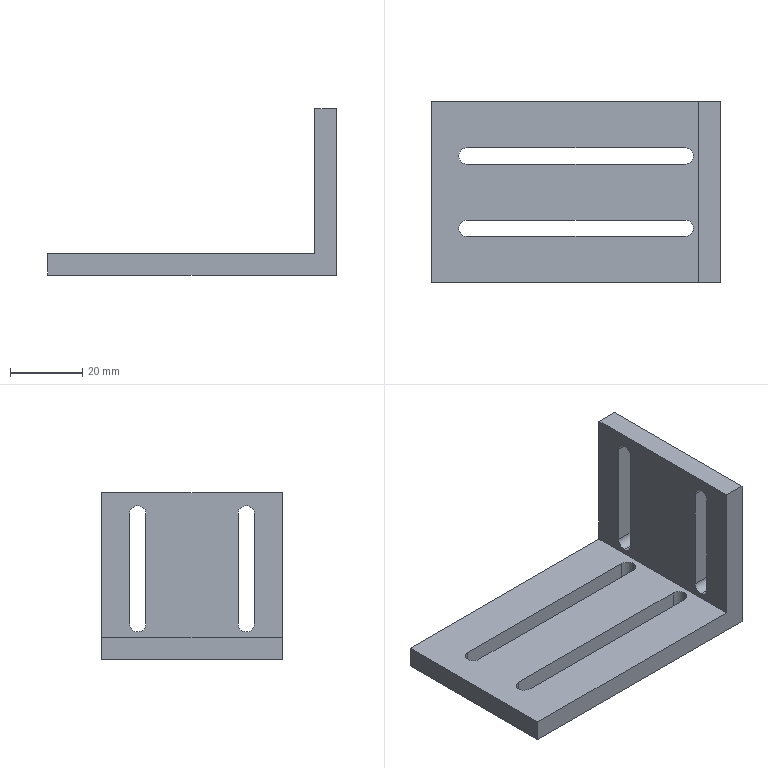Part | SolidWorks | features HoleWzd 2, Extrusion 1, ICE 1 | 1 solid | 28 faces | box 80 x 50 x 46 mm | volume 30704 mm3 | plane 16 | cylinder 12 | commonest cylinder face diameters 4.5 x12
STEP:
#1=CARTESIAN_POINT('',(34.,-15.,7.5));
#2=VERTEX_POINT('',#1);
#3=CARTESIAN_POINT('',(34.,-12.75,9.75));
#4=VERTEX_POINT('',#3);
#5=CARTESIAN_POINT('',(34.,-15.,9.75));
#6=DIRECTION('',(1.,0.,0.));
#7=DIRECTION('',(0.,0.,-1.));
#8=AXIS2_PLACEMENT_3D('',#5,#6,#7);
#9=CIRCLE('',#8,2.25);
#10=EDGE_CURVE('',#2,#4,#9,.T.);
#11=ORIENTED_EDGE('',*,*,#10,.F.);
#12=CARTESIAN_POINT('',(40.,-15.,7.5));
#13=VERTEX_POINT('',#12);
#14=CARTESIAN_POINT('',(40.,-15.,7.5));
#15=DIRECTION('',(1.,0.,0.));
#16=VECTOR('',#15,1000.);
#17=LINE('',#14,#16);
#18=EDGE_CURVE('',#2,#13,#17,.T.);
#19=ORIENTED_EDGE('',*,*,#18,.T.);
#20=CARTESIAN_POINT('',(40.,-12.75,9.75));
#21=VERTEX_POINT('',#20);
#22=CARTESIAN_POINT('',(40.,-15.,9.75));
#23=DIRECTION('',(1.,0.,0.));
#24=DIRECTION('',(0.,0.,-1.));
#25=AXIS2_PLACEMENT_3D('',#22,#23,#24);
#26=CIRCLE('',#25,2.25);
#27=EDGE_CURVE('',#13,#21,#26,.T.);
#28=ORIENTED_EDGE('',*,*,#27,.T.);
#29=CARTESIAN_POINT('',(-40.,-12.75,9.75));
#30=DIRECTION('',(-1.,0.,0.));
#31=VECTOR('',#30,1000.);
#32=LINE('',#29,#31);
#33=EDGE_CURVE('',#21,#4,#32,.T.);
#34=ORIENTED_EDGE('',*,*,#33,.T.);
#35=EDGE_LOOP('',(#11,#19,#28,#34));
#36=FACE_OUTER_BOUND('',#35,.T.);
#37=CARTESIAN_POINT('',(40.,-15.,9.75));
#38=DIRECTION('',(1.,0.,0.));
#39=DIRECTION('',(0.,0.,-1.));
#40=AXIS2_PLACEMENT_3D('',#37,#38,#39);
#41=CYLINDRICAL_SURFACE('',#40,2.25);
#42=ADVANCED_FACE('',(#36),#41,.F.);
#43=CARTESIAN_POINT('',(34.,15.,7.5));
#44=VERTEX_POINT('',#43);
#45=CARTESIAN_POINT('',(34.,17.25,9.75));
#46=VERTEX_POINT('',#45);
#47=CARTESIAN_POINT('',(34.,15.,9.75));
#48=DIRECTION('',(1.,0.,0.));
#49=DIRECTION('',(0.,0.,-1.));
#50=AXIS2_PLACEMENT_3D('',#47,#48,#49);
#51=CIRCLE('',#50,2.25);
#52=EDGE_CURVE('',#44,#46,#51,.T.);
#53=ORIENTED_EDGE('',*,*,#52,.F.);
#54=CARTESIAN_POINT('',(40.,15.,7.5));
#55=VERTEX_POINT('',#54);
#56=CARTESIAN_POINT('',(40.,15.,7.5));
#57=DIRECTION('',(1.,0.,0.));
#58=VECTOR('',#57,1000.);
#59=LINE('',#56,#58);
#60=EDGE_CURVE('',#44,#55,#59,.T.);
#61=ORIENTED_EDGE('',*,*,#60,.T.);
#62=CARTESIAN_POINT('',(40.,17.25,9.75));
#63=VERTEX_POINT('',#62);
#64=CARTESIAN_POINT('',(40.,15.,9.75));
#65=DIRECTION('',(1.,0.,0.));
#66=DIRECTION('',(0.,0.,-1.));
#67=AXIS2_PLACEMENT_3D('',#64,#65,#66);
#68=CIRCLE('',#67,2.25);
#69=EDGE_CURVE('',#55,#63,#68,.T.);
#70=ORIENTED_EDGE('',*,*,#69,.T.);
#71=CARTESIAN_POINT('',(-40.,17.25,9.75));
#72=DIRECTION('',(-1.,0.,0.));
#73=VECTOR('',#72,1000.);
#74=LINE('',#71,#73);
#75=EDGE_CURVE('',#63,#46,#74,.T.);
#76=ORIENTED_EDGE('',*,*,#75,.T.);
#77=EDGE_LOOP('',(#53,#61,#70,#76));
#78=FACE_OUTER_BOUND('',#77,.T.);
#79=CARTESIAN_POINT('',(40.,15.,9.75));
#80=DIRECTION('',(1.,0.,0.));
#81=DIRECTION('',(0.,0.,-1.));
#82=AXIS2_PLACEMENT_3D('',#79,#80,#81);
#83=CYLINDRICAL_SURFACE('',#82,2.25);
#84=ADVANCED_FACE('',(#78),#83,.F.);
#85=CARTESIAN_POINT('',(32.5,-10.,0.));
#86=VERTEX_POINT('',#85);
#87=CARTESIAN_POINT('',(30.25,-7.75,0.));
#88=VERTEX_POINT('',#87);
#89=CARTESIAN_POINT('',(30.25,-10.,0.));
#90=DIRECTION('',(0.,0.,1.));
#91=DIRECTION('',(1.,0.,0.));
#92=AXIS2_PLACEMENT_3D('',#89,#90,#91);
#93=CIRCLE('',#92,2.25);
#94=EDGE_CURVE('',#86,#88,#93,.T.);
#95=ORIENTED_EDGE('',*,*,#94,.F.);
#96=CARTESIAN_POINT('',(32.5,-10.,6.));
#97=VERTEX_POINT('',#96);
#98=CARTESIAN_POINT('',(32.5,-10.,6.));
#99=DIRECTION('',(0.,0.,1.));
#100=VECTOR('',#99,1000.);
#101=LINE('',#98,#100);
#102=EDGE_CURVE('',#86,#97,#101,.T.);
#103=ORIENTED_EDGE('',*,*,#102,.T.);
#104=CARTESIAN_POINT('',(30.25,-7.75,6.));
#105=VERTEX_POINT('',#104);
#106=CARTESIAN_POINT('',(30.25,-10.,6.));
#107=DIRECTION('',(0.,0.,1.));
#108=DIRECTION('',(1.,0.,0.));
#109=AXIS2_PLACEMENT_3D('',#106,#107,#108);
#110=CIRCLE('',#109,2.25);
#111=EDGE_CURVE('',#97,#105,#110,.T.);
#112=ORIENTED_EDGE('',*,*,#111,.T.);
#113=CARTESIAN_POINT('',(30.25,-7.75,6.));
#114=DIRECTION('',(0.,0.,1.));
#115=VECTOR('',#114,1000.);
#116=LINE('',#113,#115);
#117=EDGE_CURVE('',#88,#105,#116,.T.);
#118=ORIENTED_EDGE('',*,*,#117,.F.);
#119=EDGE_LOOP('',(#95,#103,#112,#118));
#120=FACE_OUTER_BOUND('',#119,.T.);
#121=CARTESIAN_POINT('',(30.25,-10.,6.));
#122=DIRECTION('',(0.,0.,1.));
#123=DIRECTION('',(1.,0.,0.));
#124=AXIS2_PLACEMENT_3D('',#121,#122,#123);
#125=CYLINDRICAL_SURFACE('',#124,2.25);
#126=ADVANCED_FACE('',(#120),#125,.F.);
#127=CARTESIAN_POINT('',(32.5,10.,0.));
#128=VERTEX_POINT('',#127);
#129=CARTESIAN_POINT('',(30.25,12.25,0.));
#130=VERTEX_POINT('',#129);
#131=CARTESIAN_POINT('',(30.25,10.,0.));
#132=DIRECTION('',(0.,0.,1.));
#133=DIRECTION('',(1.,0.,0.));
#134=AXIS2_PLACEMENT_3D('',#131,#132,#133);
#135=CIRCLE('',#134,2.25);
#136=EDGE_CURVE('',#128,#130,#135,.T.);
#137=ORIENTED_EDGE('',*,*,#136,.F.);
#138=CARTESIAN_POINT('',(32.5,10.,6.));
#139=VERTEX_POINT('',#138);
#140=CARTESIAN_POINT('',(32.5,10.,6.));
#141=DIRECTION('',(0.,0.,1.));
#142=VECTOR('',#141,1000.);
#143=LINE('',#140,#142);
#144=EDGE_CURVE('',#128,#139,#143,.T.);
#145=ORIENTED_EDGE('',*,*,#144,.T.);
#146=CARTESIAN_POINT('',(30.25,12.25,6.));
#147=VERTEX_POINT('',#146);
#148=CARTESIAN_POINT('',(30.25,10.,6.));
#149=DIRECTION('',(0.,0.,1.));
#150=DIRECTION('',(1.,0.,0.));
#151=AXIS2_PLACEMENT_3D('',#148,#149,#150);
#152=CIRCLE('',#151,2.25);
#153=EDGE_CURVE('',#139,#147,#152,.T.);
#154=ORIENTED_EDGE('',*,*,#153,.T.);
#155=CARTESIAN_POINT('',(30.25,12.25,6.));
#156=DIRECTION('',(0.,0.,1.));
#157=VECTOR('',#156,1000.);
#158=LINE('',#155,#157);
#159=EDGE_CURVE('',#130,#147,#158,.T.);
#160=ORIENTED_EDGE('',*,*,#159,.F.);
#161=EDGE_LOOP('',(#137,#145,#154,#160));
#162=FACE_OUTER_BOUND('',#161,.T.);
#163=CARTESIAN_POINT('',(30.25,10.,6.));
#164=DIRECTION('',(0.,0.,1.));
#165=DIRECTION('',(1.,0.,0.));
#166=AXIS2_PLACEMENT_3D('',#163,#164,#165);
#167=CYLINDRICAL_SURFACE('',#166,2.25);
#168=ADVANCED_FACE('',(#162),#167,.F.);
#169=CARTESIAN_POINT('',(40.,-25.,0.));
#170=VERTEX_POINT('',#169);
#171=CARTESIAN_POINT('',(40.,25.,0.));
#172=VERTEX_POINT('',#171);
#173=CARTESIAN_POINT('',(40.,25.,0.));
#174=DIRECTION('',(0.,1.,0.));
#175=VECTOR('',#174,1000.);
#176=LINE('',#173,#175);
#177=EDGE_CURVE('',#170,#172,#176,.T.);
#178=ORIENTED_EDGE('',*,*,#177,.T.);
#179=CARTESIAN_POINT('',(40.,25.,46.));
#180=VERTEX_POINT('',#179);
#181=CARTESIAN_POINT('',(40.,25.,6.));
#182=DIRECTION('',(0.,0.,-1.));
#183=VECTOR('',#182,1000.);
#184=LINE('',#181,#183);
#185=EDGE_CURVE('',#180,#172,#184,.T.);
#186=ORIENTED_EDGE('',*,*,#185,.F.);
#187=CARTESIAN_POINT('',(40.,-25.,46.));
#188=VERTEX_POINT('',#187);
#189=CARTESIAN_POINT('',(40.,25.,46.));
#190=DIRECTION('',(0.,1.,0.));
#191=VECTOR('',#190,1000.);
#192=LINE('',#189,#191);
#193=EDGE_CURVE('',#188,#180,#192,.T.);
#194=ORIENTED_EDGE('',*,*,#193,.F.);
#195=CARTESIAN_POINT('',(40.,-25.,6.));
#196=DIRECTION('',(0.,0.,-1.));
#197=VECTOR('',#196,1000.);
#198=LINE('',#195,#197);
#199=EDGE_CURVE('',#188,#170,#198,.T.);
#200=ORIENTED_EDGE('',*,*,#199,.T.);
#201=EDGE_LOOP('',(#178,#186,#194,#200));
#202=FACE_OUTER_BOUND('',#201,.T.);
#203=CARTESIAN_POINT('',(40.,12.75,9.75));
#204=VERTEX_POINT('',#203);
#205=CARTESIAN_POINT('',(40.,15.,9.75));
#206=DIRECTION('',(1.,0.,0.));
#207=DIRECTION('',(0.,0.,-1.));
#208=AXIS2_PLACEMENT_3D('',#205,#206,#207);
#209=CIRCLE('',#208,2.25);
#210=EDGE_CURVE('',#204,#55,#209,.T.);
#211=ORIENTED_EDGE('',*,*,#210,.F.);
#212=CARTESIAN_POINT('',(40.,12.75,40.25));
#213=VERTEX_POINT('',#212);
#214=CARTESIAN_POINT('',(40.,12.75,9.75));
#215=DIRECTION('',(0.,0.,1.));
#216=VECTOR('',#215,1000.);
#217=LINE('',#214,#216);
#218=EDGE_CURVE('',#204,#213,#217,.T.);
#219=ORIENTED_EDGE('',*,*,#218,.T.);
#220=CARTESIAN_POINT('',(40.,17.25,40.25));
#221=VERTEX_POINT('',#220);
#222=CARTESIAN_POINT('',(40.,15.,40.25));
#223=DIRECTION('',(1.,0.,0.));
#224=DIRECTION('',(0.,0.,-1.));
#225=AXIS2_PLACEMENT_3D('',#222,#223,#224);
#226=CIRCLE('',#225,2.25);
#227=EDGE_CURVE('',#221,#213,#226,.T.);
#228=ORIENTED_EDGE('',*,*,#227,.F.);
#229=CARTESIAN_POINT('',(40.,17.25,9.75));
#230=DIRECTION('',(0.,0.,1.));
#231=VECTOR('',#230,1000.);
#232=LINE('',#229,#231);
#233=EDGE_CURVE('',#63,#221,#232,.T.);
#234=ORIENTED_EDGE('',*,*,#233,.F.);
#235=ORIENTED_EDGE('',*,*,#69,.F.);
#236=EDGE_LOOP('',(#211,#219,#228,#234,#235));
#237=FACE_BOUND('',#236,.T.);
#238=CARTESIAN_POINT('',(40.,-12.75,40.25));
#239=VERTEX_POINT('',#238);
#240=CARTESIAN_POINT('',(40.,-12.75,9.75));
#241=DIRECTION('',(0.,0.,1.));
#242=VECTOR('',#241,1000.);
#243=LINE('',#240,#242);
#244=EDGE_CURVE('',#21,#239,#243,.T.);
#245=ORIENTED_EDGE('',*,*,#244,.F.);
#246=ORIENTED_EDGE('',*,*,#27,.F.);
#247=CARTESIAN_POINT('',(40.,-17.25,9.75));
#248=VERTEX_POINT('',#247);
#249=CARTESIAN_POINT('',(40.,-15.,9.75));
#250=DIRECTION('',(1.,0.,0.));
#251=DIRECTION('',(0.,0.,-1.));
#252=AXIS2_PLACEMENT_3D('',#249,#250,#251);
#253=CIRCLE('',#252,2.25);
#254=EDGE_CURVE('',#248,#13,#253,.T.);
#255=ORIENTED_EDGE('',*,*,#254,.F.);
#256=CARTESIAN_POINT('',(40.,-17.25,40.25));
#257=VERTEX_POINT('',#256);
#258=CARTESIAN_POINT('',(40.,-17.25,9.75));
#259=DIRECTION('',(0.,0.,1.));
#260=VECTOR('',#259,1000.);
#261=LINE('',#258,#260);
#262=EDGE_CURVE('',#248,#257,#261,.T.);
#263=ORIENTED_EDGE('',*,*,#262,.T.);
#264=CARTESIAN_POINT('',(40.,-15.,40.25));
#265=DIRECTION('',(1.,0.,0.));
#266=DIRECTION('',(0.,0.,-1.));
#267=AXIS2_PLACEMENT_3D('',#264,#265,#266);
#268=CIRCLE('',#267,2.25);
#269=EDGE_CURVE('',#239,#257,#268,.T.);
#270=ORIENTED_EDGE('',*,*,#269,.F.);
#271=EDGE_LOOP('',(#245,#246,#255,#263,#270));
#272=FACE_BOUND('',#271,.T.);
#273=CARTESIAN_POINT('',(40.,25.,6.));
#274=DIRECTION('',(-1.,0.,0.));
#275=DIRECTION('',(0.,-1.,0.));
#276=AXIS2_PLACEMENT_3D('',#273,#274,#275);
#277=PLANE('',#276);
#278=ADVANCED_FACE('',(#202,#237,#272),#277,.F.);
#279=CARTESIAN_POINT('',(-40.,25.,0.));
#280=VERTEX_POINT('',#279);
#281=CARTESIAN_POINT('',(-40.,25.,0.));
#282=DIRECTION('',(-1.,0.,0.));
#283=VECTOR('',#282,1000.);
#284=LINE('',#281,#283);
#285=EDGE_CURVE('',#172,#280,#284,.T.);
#286=ORIENTED_EDGE('',*,*,#285,.T.);
#287=CARTESIAN_POINT('',(-40.,25.,6.));
#288=VERTEX_POINT('',#287);
#289=CARTESIAN_POINT('',(-40.,25.,6.));
#290=DIRECTION('',(0.,0.,-1.));
#291=VECTOR('',#290,1000.);
#292=LINE('',#289,#291);
#293=EDGE_CURVE('',#288,#280,#292,.T.);
#294=ORIENTED_EDGE('',*,*,#293,.F.);
#295=CARTESIAN_POINT('',(34.,25.,6.));
#296=VERTEX_POINT('',#295);
#297=CARTESIAN_POINT('',(-40.,25.,6.));
#298=DIRECTION('',(-1.,0.,0.));
#299=VECTOR('',#298,1000.);
#300=LINE('',#297,#299);
#301=EDGE_CURVE('',#296,#288,#300,.T.);
#302=ORIENTED_EDGE('',*,*,#301,.F.);
#303=CARTESIAN_POINT('',(34.,25.,46.));
#304=VERTEX_POINT('',#303);
#305=CARTESIAN_POINT('',(34.,25.,46.));
#306=DIRECTION('',(0.,0.,-1.));
#307=VECTOR('',#306,1000.);
#308=LINE('',#305,#307);
#309=EDGE_CURVE('',#304,#296,#308,.T.);
#310=ORIENTED_EDGE('',*,*,#309,.F.);
#311=CARTESIAN_POINT('',(40.,25.,46.));
#312=DIRECTION('',(-1.,0.,0.));
#313=VECTOR('',#312,1000.);
#314=LINE('',#311,#313);
#315=EDGE_CURVE('',#180,#304,#314,.T.);
#316=ORIENTED_EDGE('',*,*,#315,.F.);
#317=ORIENTED_EDGE('',*,*,#185,.T.);
#318=EDGE_LOOP('',(#286,#294,#302,#310,#316,#317));
#319=FACE_OUTER_BOUND('',#318,.T.);
#320=CARTESIAN_POINT('',(-40.,25.,6.));
#321=DIRECTION('',(0.,-1.,0.));
#322=DIRECTION('',(0.,0.,-1.));
#323=AXIS2_PLACEMENT_3D('',#320,#321,#322);
#324=PLANE('',#323);
#325=ADVANCED_FACE('',(#319),#324,.F.);
#326=CARTESIAN_POINT('',(-40.,-25.,0.));
#327=VERTEX_POINT('',#326);
#328=CARTESIAN_POINT('',(-40.,25.,0.));
#329=DIRECTION('',(0.,-1.,0.));
#330=VECTOR('',#329,1000.);
#331=LINE('',#328,#330);
#332=EDGE_CURVE('',#280,#327,#331,.T.);
#333=ORIENTED_EDGE('',*,*,#332,.T.);
#334=CARTESIAN_POINT('',(-40.,-25.,6.));
#335=VERTEX_POINT('',#334);
#336=CARTESIAN_POINT('',(-40.,-25.,6.));
#337=DIRECTION('',(0.,0.,-1.));
#338=VECTOR('',#337,1000.);
#339=LINE('',#336,#338);
#340=EDGE_CURVE('',#335,#327,#339,.T.);
#341=ORIENTED_EDGE('',*,*,#340,.F.);
#342=CARTESIAN_POINT('',(-40.,25.,6.));
#343=DIRECTION('',(0.,-1.,0.));
#344=VECTOR('',#343,1000.);
#345=LINE('',#342,#344);
#346=EDGE_CURVE('',#288,#335,#345,.T.);
#347=ORIENTED_EDGE('',*,*,#346,.F.);
#348=ORIENTED_EDGE('',*,*,#293,.T.);
#349=EDGE_LOOP('',(#333,#341,#347,#348));
#350=FACE_OUTER_BOUND('',#349,.T.);
#351=CARTESIAN_POINT('',(-40.,25.,6.));
#352=DIRECTION('',(1.,0.,0.));
#353=DIRECTION('',(0.,1.,0.));
#354=AXIS2_PLACEMENT_3D('',#351,#352,#353);
#355=PLANE('',#354);
#356=ADVANCED_FACE('',(#350),#355,.F.);
#357=CARTESIAN_POINT('',(-40.,-25.,0.));
#358=DIRECTION('',(1.,0.,0.));
#359=VECTOR('',#358,1000.);
#360=LINE('',#357,#359);
#361=EDGE_CURVE('',#327,#170,#360,.T.);
#362=ORIENTED_EDGE('',*,*,#361,.T.);
#363=ORIENTED_EDGE('',*,*,#199,.F.);
#364=CARTESIAN_POINT('',(34.,-25.,46.));
#365=VERTEX_POINT('',#364);
#366=CARTESIAN_POINT('',(40.,-25.,46.));
#367=DIRECTION('',(1.,0.,0.));
#368=VECTOR('',#367,1000.);
#369=LINE('',#366,#368);
#370=EDGE_CURVE('',#365,#188,#369,.T.);
#371=ORIENTED_EDGE('',*,*,#370,.F.);
#372=CARTESIAN_POINT('',(34.,-25.,6.));
#373=VERTEX_POINT('',#372);
#374=CARTESIAN_POINT('',(34.,-25.,46.));
#375=DIRECTION('',(0.,0.,-1.));
#376=VECTOR('',#375,1000.);
#377=LINE('',#374,#376);
#378=EDGE_CURVE('',#365,#373,#377,.T.);
#379=ORIENTED_EDGE('',*,*,#378,.T.);
#380=CARTESIAN_POINT('',(-40.,-25.,6.));
#381=DIRECTION('',(1.,0.,0.));
#382=VECTOR('',#381,1000.);
#383=LINE('',#380,#382);
#384=EDGE_CURVE('',#335,#373,#383,.T.);
#385=ORIENTED_EDGE('',*,*,#384,.F.);
#386=ORIENTED_EDGE('',*,*,#340,.T.);
#387=EDGE_LOOP('',(#362,#363,#371,#379,#385,#386));
#388=FACE_OUTER_BOUND('',#387,.T.);
#389=CARTESIAN_POINT('',(-40.,-25.,6.));
#390=DIRECTION('',(0.,1.,0.));
#391=DIRECTION('',(0.,0.,1.));
#392=AXIS2_PLACEMENT_3D('',#389,#390,#391);
#393=PLANE('',#392);
#394=ADVANCED_FACE('',(#388),#393,.F.);
#395=CARTESIAN_POINT('',(34.,25.,6.));
#396=DIRECTION('',(0.,-1.,0.));
#397=VECTOR('',#396,1000.);
#398=LINE('',#395,#397);
#399=EDGE_CURVE('',#296,#373,#398,.T.);
#400=ORIENTED_EDGE('',*,*,#399,.F.);
#401=ORIENTED_EDGE('',*,*,#301,.T.);
#402=ORIENTED_EDGE('',*,*,#346,.T.);
#403=ORIENTED_EDGE('',*,*,#384,.T.);
#404=EDGE_LOOP('',(#400,#401,#402,#403));
#405=FACE_OUTER_BOUND('',#404,.T.);
#406=CARTESIAN_POINT('',(30.25,-12.25,6.));
#407=VERTEX_POINT('',#406);
#408=CARTESIAN_POINT('',(30.25,-10.,6.));
#409=DIRECTION('',(0.,0.,1.));
#410=DIRECTION('',(1.,0.,0.));
#411=AXIS2_PLACEMENT_3D('',#408,#409,#410);
#412=CIRCLE('',#411,2.25);
#413=EDGE_CURVE('',#407,#97,#412,.T.);
#414=ORIENTED_EDGE('',*,*,#413,.F.);
#415=CARTESIAN_POINT('',(-30.25,-12.25,6.));
#416=VERTEX_POINT('',#415);
#417=CARTESIAN_POINT('',(-30.25,-12.25,6.));
#418=DIRECTION('',(1.,0.,0.));
#419=VECTOR('',#418,1000.);
#420=LINE('',#417,#419);
#421=EDGE_CURVE('',#416,#407,#420,.T.);
#422=ORIENTED_EDGE('',*,*,#421,.F.);
#423=CARTESIAN_POINT('',(-30.25,-7.75,6.));
#424=VERTEX_POINT('',#423);
#425=CARTESIAN_POINT('',(-30.25,-10.,6.));
#426=DIRECTION('',(0.,0.,1.));
#427=DIRECTION('',(1.,0.,0.));
#428=AXIS2_PLACEMENT_3D('',#425,#426,#427);
#429=CIRCLE('',#428,2.25);
#430=EDGE_CURVE('',#424,#416,#429,.T.);
#431=ORIENTED_EDGE('',*,*,#430,.F.);
#432=CARTESIAN_POINT('',(-30.25,-7.75,6.));
#433=DIRECTION('',(1.,0.,0.));
#434=VECTOR('',#433,1000.);
#435=LINE('',#432,#434);
#436=EDGE_CURVE('',#424,#105,#435,.T.);
#437=ORIENTED_EDGE('',*,*,#436,.T.);
#438=ORIENTED_EDGE('',*,*,#111,.F.);
#439=EDGE_LOOP('',(#414,#422,#431,#437,#438));
#440=FACE_BOUND('',#439,.T.);
#441=CARTESIAN_POINT('',(-30.25,7.75,6.));
#442=VERTEX_POINT('',#441);
#443=CARTESIAN_POINT('',(30.25,7.75,6.));
#444=VERTEX_POINT('',#443);
#445=CARTESIAN_POINT('',(-30.25,7.75,6.));
#446=DIRECTION('',(1.,0.,0.));
#447=VECTOR('',#446,1000.);
#448=LINE('',#445,#447);
#449=EDGE_CURVE('',#442,#444,#448,.T.);
#450=ORIENTED_EDGE('',*,*,#449,.F.);
#451=CARTESIAN_POINT('',(-30.25,12.25,6.));
#452=VERTEX_POINT('',#451);
#453=CARTESIAN_POINT('',(-30.25,10.,6.));
#454=DIRECTION('',(0.,0.,1.));
#455=DIRECTION('',(1.,0.,0.));
#456=AXIS2_PLACEMENT_3D('',#453,#454,#455);
#457=CIRCLE('',#456,2.25);
#458=EDGE_CURVE('',#452,#442,#457,.T.);
#459=ORIENTED_EDGE('',*,*,#458,.F.);
#460=CARTESIAN_POINT('',(-30.25,12.25,6.));
#461=DIRECTION('',(1.,0.,0.));
#462=VECTOR('',#461,1000.);
#463=LINE('',#460,#462);
#464=EDGE_CURVE('',#452,#147,#463,.T.);
#465=ORIENTED_EDGE('',*,*,#464,.T.);
#466=ORIENTED_EDGE('',*,*,#153,.F.);
#467=CARTESIAN_POINT('',(30.25,10.,6.));
#468=DIRECTION('',(0.,0.,1.));
#469=DIRECTION('',(1.,0.,0.));
#470=AXIS2_PLACEMENT_3D('',#467,#468,#469);
#471=CIRCLE('',#470,2.25);
#472=EDGE_CURVE('',#444,#139,#471,.T.);
#473=ORIENTED_EDGE('',*,*,#472,.F.);
#474=EDGE_LOOP('',(#450,#459,#465,#466,#473));
#475=FACE_BOUND('',#474,.T.);
#476=CARTESIAN_POINT('',(0.,0.,6.));
#477=DIRECTION('',(0.,0.,1.));
#478=DIRECTION('',(1.,0.,0.));
#479=AXIS2_PLACEMENT_3D('',#476,#477,#478);
#480=PLANE('',#479);
#481=ADVANCED_FACE('',(#405,#440,#475),#480,.T.);
#482=CARTESIAN_POINT('',(-30.25,-12.25,0.));
#483=VERTEX_POINT('',#482);
#484=CARTESIAN_POINT('',(30.25,-12.25,0.));
#485=VERTEX_POINT('',#484);
#486=CARTESIAN_POINT('',(-30.25,-12.25,0.));
#487=DIRECTION('',(1.,0.,0.));
#488=VECTOR('',#487,1000.);
#489=LINE('',#486,#488);
#490=EDGE_CURVE('',#483,#485,#489,.T.);
#491=ORIENTED_EDGE('',*,*,#490,.T.);
#492=CARTESIAN_POINT('',(30.25,-10.,0.));
#493=DIRECTION('',(0.,0.,1.));
#494=DIRECTION('',(1.,0.,0.));
#495=AXIS2_PLACEMENT_3D('',#492,#493,#494);
#496=CIRCLE('',#495,2.25);
#497=EDGE_CURVE('',#485,#86,#496,.T.);
#498=ORIENTED_EDGE('',*,*,#497,.T.);
#499=ORIENTED_EDGE('',*,*,#94,.T.);
#500=CARTESIAN_POINT('',(-30.25,-7.75,0.));
#501=VERTEX_POINT('',#500);
#502=CARTESIAN_POINT('',(-30.25,-7.75,0.));
#503=DIRECTION('',(1.,0.,0.));
#504=VECTOR('',#503,1000.);
#505=LINE('',#502,#504);
#506=EDGE_CURVE('',#501,#88,#505,.T.);
#507=ORIENTED_EDGE('',*,*,#506,.F.);
#508=CARTESIAN_POINT('',(-30.25,-10.,0.));
#509=DIRECTION('',(0.,0.,1.));
#510=DIRECTION('',(1.,0.,0.));
#511=AXIS2_PLACEMENT_3D('',#508,#509,#510);
#512=CIRCLE('',#511,2.25);
#513=EDGE_CURVE('',#501,#483,#512,.T.);
#514=ORIENTED_EDGE('',*,*,#513,.T.);
#515=EDGE_LOOP('',(#491,#498,#499,#507,#514));
#516=FACE_BOUND('',#515,.T.);
#517=CARTESIAN_POINT('',(-30.25,7.75,0.));
#518=VERTEX_POINT('',#517);
#519=CARTESIAN_POINT('',(30.25,7.75,0.));
#520=VERTEX_POINT('',#519);
#521=CARTESIAN_POINT('',(-30.25,7.75,0.));
#522=DIRECTION('',(1.,0.,0.));
#523=VECTOR('',#522,1000.);
#524=LINE('',#521,#523);
#525=EDGE_CURVE('',#518,#520,#524,.T.);
#526=ORIENTED_EDGE('',*,*,#525,.T.);
#527=CARTESIAN_POINT('',(30.25,10.,0.));
#528=DIRECTION('',(0.,0.,1.));
#529=DIRECTION('',(1.,0.,0.));
#530=AXIS2_PLACEMENT_3D('',#527,#528,#529);
#531=CIRCLE('',#530,2.25);
#532=EDGE_CURVE('',#520,#128,#531,.T.);
#533=ORIENTED_EDGE('',*,*,#532,.T.);
#534=ORIENTED_EDGE('',*,*,#136,.T.);
#535=CARTESIAN_POINT('',(-30.25,12.25,0.));
#536=VERTEX_POINT('',#535);
#537=CARTESIAN_POINT('',(-30.25,12.25,0.));
#538=DIRECTION('',(1.,0.,0.));
#539=VECTOR('',#538,1000.);
#540=LINE('',#537,#539);
#541=EDGE_CURVE('',#536,#130,#540,.T.);
#542=ORIENTED_EDGE('',*,*,#541,.F.);
#543=CARTESIAN_POINT('',(-30.25,10.,0.));
#544=DIRECTION('',(0.,0.,1.));
#545=DIRECTION('',(1.,0.,0.));
#546=AXIS2_PLACEMENT_3D('',#543,#544,#545);
#547=CIRCLE('',#546,2.25);
#548=EDGE_CURVE('',#536,#518,#547,.T.);
#549=ORIENTED_EDGE('',*,*,#548,.T.);
#550=EDGE_LOOP('',(#526,#533,#534,#542,#549));
#551=FACE_BOUND('',#550,.T.);
#552=ORIENTED_EDGE('',*,*,#177,.F.);
#553=ORIENTED_EDGE('',*,*,#361,.F.);
#554=ORIENTED_EDGE('',*,*,#332,.F.);
#555=ORIENTED_EDGE('',*,*,#285,.F.);
#556=EDGE_LOOP('',(#552,#553,#554,#555));
#557=FACE_OUTER_BOUND('',#556,.T.);
#558=CARTESIAN_POINT('',(0.,0.,0.));
#559=DIRECTION('',(0.,0.,1.));
#560=DIRECTION('',(1.,0.,0.));
#561=AXIS2_PLACEMENT_3D('',#558,#559,#560);
#562=PLANE('',#561);
#563=ADVANCED_FACE('',(#516,#551,#557),#562,.F.);
#564=ORIENTED_EDGE('',*,*,#144,.F.);
#565=ORIENTED_EDGE('',*,*,#532,.F.);
#566=CARTESIAN_POINT('',(30.25,7.75,6.));
#567=DIRECTION('',(0.,0.,-1.));
#568=VECTOR('',#567,1000.);
#569=LINE('',#566,#568);
#570=EDGE_CURVE('',#444,#520,#569,.T.);
#571=ORIENTED_EDGE('',*,*,#570,.F.);
#572=ORIENTED_EDGE('',*,*,#472,.T.);
#573=EDGE_LOOP('',(#564,#565,#571,#572));
#574=FACE_OUTER_BOUND('',#573,.T.);
#575=CARTESIAN_POINT('',(30.25,10.,6.));
#576=DIRECTION('',(0.,0.,1.));
#577=DIRECTION('',(1.,0.,0.));
#578=AXIS2_PLACEMENT_3D('',#575,#576,#577);
#579=CYLINDRICAL_SURFACE('',#578,2.25);
#580=ADVANCED_FACE('',(#574),#579,.F.);
#581=ORIENTED_EDGE('',*,*,#458,.T.);
#582=CARTESIAN_POINT('',(-30.25,7.75,6.));
#583=DIRECTION('',(0.,0.,1.));
#584=VECTOR('',#583,1000.);
#585=LINE('',#582,#584);
#586=EDGE_CURVE('',#518,#442,#585,.T.);
#587=ORIENTED_EDGE('',*,*,#586,.F.);
#588=ORIENTED_EDGE('',*,*,#548,.F.);
#589=CARTESIAN_POINT('',(-30.25,12.25,6.));
#590=DIRECTION('',(0.,0.,-1.));
#591=VECTOR('',#590,1000.);
#592=LINE('',#589,#591);
#593=EDGE_CURVE('',#452,#536,#592,.T.);
#594=ORIENTED_EDGE('',*,*,#593,.F.);
#595=EDGE_LOOP('',(#581,#587,#588,#594));
#596=FACE_OUTER_BOUND('',#595,.T.);
#597=CARTESIAN_POINT('',(-30.25,10.,6.));
#598=DIRECTION('',(0.,0.,1.));
#599=DIRECTION('',(1.,0.,0.));
#600=AXIS2_PLACEMENT_3D('',#597,#598,#599);
#601=CYLINDRICAL_SURFACE('',#600,2.25);
#602=ADVANCED_FACE('',(#596),#601,.F.);
#603=ORIENTED_EDGE('',*,*,#159,.T.);
#604=ORIENTED_EDGE('',*,*,#464,.F.);
#605=ORIENTED_EDGE('',*,*,#593,.T.);
#606=ORIENTED_EDGE('',*,*,#541,.T.);
#607=EDGE_LOOP('',(#603,#604,#605,#606));
#608=FACE_OUTER_BOUND('',#607,.T.);
#609=CARTESIAN_POINT('',(-30.25,12.25,6.));
#610=DIRECTION('',(0.,1.,0.));
#611=DIRECTION('',(-1.,0.,0.));
#612=AXIS2_PLACEMENT_3D('',#609,#610,#611);
#613=PLANE('',#612);
#614=ADVANCED_FACE('',(#608),#613,.F.);
#615=ORIENTED_EDGE('',*,*,#570,.T.);
#616=ORIENTED_EDGE('',*,*,#525,.F.);
#617=ORIENTED_EDGE('',*,*,#586,.T.);
#618=ORIENTED_EDGE('',*,*,#449,.T.);
#619=EDGE_LOOP('',(#615,#616,#617,#618));
#620=FACE_OUTER_BOUND('',#619,.T.);
#621=CARTESIAN_POINT('',(-30.25,7.75,6.));
#622=DIRECTION('',(0.,-1.,0.));
#623=DIRECTION('',(1.,0.,0.));
#624=AXIS2_PLACEMENT_3D('',#621,#622,#623);
#625=PLANE('',#624);
#626=ADVANCED_FACE('',(#620),#625,.F.);
#627=ORIENTED_EDGE('',*,*,#102,.F.);
#628=ORIENTED_EDGE('',*,*,#497,.F.);
#629=CARTESIAN_POINT('',(30.25,-12.25,6.));
#630=DIRECTION('',(0.,0.,-1.));
#631=VECTOR('',#630,1000.);
#632=LINE('',#629,#631);
#633=EDGE_CURVE('',#407,#485,#632,.T.);
#634=ORIENTED_EDGE('',*,*,#633,.F.);
#635=ORIENTED_EDGE('',*,*,#413,.T.);
#636=EDGE_LOOP('',(#627,#628,#634,#635));
#637=FACE_OUTER_BOUND('',#636,.T.);
#638=CARTESIAN_POINT('',(30.25,-10.,6.));
#639=DIRECTION('',(0.,0.,1.));
#640=DIRECTION('',(1.,0.,0.));
#641=AXIS2_PLACEMENT_3D('',#638,#639,#640);
#642=CYLINDRICAL_SURFACE('',#641,2.25);
#643=ADVANCED_FACE('',(#637),#642,.F.);
#644=ORIENTED_EDGE('',*,*,#430,.T.);
#645=CARTESIAN_POINT('',(-30.25,-12.25,6.));
#646=DIRECTION('',(0.,0.,1.));
#647=VECTOR('',#646,1000.);
#648=LINE('',#645,#647);
#649=EDGE_CURVE('',#483,#416,#648,.T.);
#650=ORIENTED_EDGE('',*,*,#649,.F.);
#651=ORIENTED_EDGE('',*,*,#513,.F.);
#652=CARTESIAN_POINT('',(-30.25,-7.75,6.));
#653=DIRECTION('',(0.,0.,-1.));
#654=VECTOR('',#653,1000.);
#655=LINE('',#652,#654);
#656=EDGE_CURVE('',#424,#501,#655,.T.);
#657=ORIENTED_EDGE('',*,*,#656,.F.);
#658=EDGE_LOOP('',(#644,#650,#651,#657));
#659=FACE_OUTER_BOUND('',#658,.T.);
#660=CARTESIAN_POINT('',(-30.25,-10.,6.));
#661=DIRECTION('',(0.,0.,1.));
#662=DIRECTION('',(1.,0.,0.));
#663=AXIS2_PLACEMENT_3D('',#660,#661,#662);
#664=CYLINDRICAL_SURFACE('',#663,2.25);
#665=ADVANCED_FACE('',(#659),#664,.F.);
#666=ORIENTED_EDGE('',*,*,#117,.T.);
#667=ORIENTED_EDGE('',*,*,#436,.F.);
#668=ORIENTED_EDGE('',*,*,#656,.T.);
#669=ORIENTED_EDGE('',*,*,#506,.T.);
#670=EDGE_LOOP('',(#666,#667,#668,#669));
#671=FACE_OUTER_BOUND('',#670,.T.);
#672=CARTESIAN_POINT('',(-30.25,-7.75,6.));
#673=DIRECTION('',(0.,1.,0.));
#674=DIRECTION('',(-1.,0.,0.));
#675=AXIS2_PLACEMENT_3D('',#672,#673,#674);
#676=PLANE('',#675);
#677=ADVANCED_FACE('',(#671),#676,.F.);
#678=ORIENTED_EDGE('',*,*,#633,.T.);
#679=ORIENTED_EDGE('',*,*,#490,.F.);
#680=ORIENTED_EDGE('',*,*,#649,.T.);
#681=ORIENTED_EDGE('',*,*,#421,.T.);
#682=EDGE_LOOP('',(#678,#679,#680,#681));
#683=FACE_OUTER_BOUND('',#682,.T.);
#684=CARTESIAN_POINT('',(-30.25,-12.25,6.));
#685=DIRECTION('',(0.,-1.,0.));
#686=DIRECTION('',(1.,0.,0.));
#687=AXIS2_PLACEMENT_3D('',#684,#685,#686);
#688=PLANE('',#687);
#689=ADVANCED_FACE('',(#683),#688,.F.);
#690=CARTESIAN_POINT('',(34.,-12.75,40.25));
#691=VERTEX_POINT('',#690);
#692=CARTESIAN_POINT('',(34.,-17.25,40.25));
#693=VERTEX_POINT('',#692);
#694=CARTESIAN_POINT('',(34.,-15.,40.25));
#695=DIRECTION('',(1.,0.,0.));
#696=DIRECTION('',(0.,0.,-1.));
#697=AXIS2_PLACEMENT_3D('',#694,#695,#696);
#698=CIRCLE('',#697,2.25);
#699=EDGE_CURVE('',#691,#693,#698,.T.);
#700=ORIENTED_EDGE('',*,*,#699,.T.);
#701=CARTESIAN_POINT('',(34.,-17.25,9.75));
#702=VERTEX_POINT('',#701);
#703=CARTESIAN_POINT('',(34.,-17.25,46.));
#704=DIRECTION('',(0.,0.,-1.));
#705=VECTOR('',#704,1000.);
#706=LINE('',#703,#705);
#707=EDGE_CURVE('',#693,#702,#706,.T.);
#708=ORIENTED_EDGE('',*,*,#707,.T.);
#709=CARTESIAN_POINT('',(34.,-15.,9.75));
#710=DIRECTION('',(1.,0.,0.));
#711=DIRECTION('',(0.,0.,-1.));
#712=AXIS2_PLACEMENT_3D('',#709,#710,#711);
#713=CIRCLE('',#712,2.25);
#714=EDGE_CURVE('',#702,#2,#713,.T.);
#715=ORIENTED_EDGE('',*,*,#714,.T.);
#716=ORIENTED_EDGE('',*,*,#10,.T.);
#717=CARTESIAN_POINT('',(34.,-12.75,46.));
#718=DIRECTION('',(0.,0.,1.));
#719=VECTOR('',#718,1000.);
#720=LINE('',#717,#719);
#721=EDGE_CURVE('',#4,#691,#720,.T.);
#722=ORIENTED_EDGE('',*,*,#721,.T.);
#723=EDGE_LOOP('',(#700,#708,#715,#716,#722));
#724=FACE_BOUND('',#723,.T.);
#725=CARTESIAN_POINT('',(34.,17.25,40.25));
#726=VERTEX_POINT('',#725);
#727=CARTESIAN_POINT('',(34.,17.25,46.));
#728=DIRECTION('',(0.,0.,1.));
#729=VECTOR('',#728,1000.);
#730=LINE('',#727,#729);
#731=EDGE_CURVE('',#46,#726,#730,.T.);
#732=ORIENTED_EDGE('',*,*,#731,.T.);
#733=CARTESIAN_POINT('',(34.,12.75,40.25));
#734=VERTEX_POINT('',#733);
#735=CARTESIAN_POINT('',(34.,15.,40.25));
#736=DIRECTION('',(1.,0.,0.));
#737=DIRECTION('',(0.,0.,-1.));
#738=AXIS2_PLACEMENT_3D('',#735,#736,#737);
#739=CIRCLE('',#738,2.25);
#740=EDGE_CURVE('',#726,#734,#739,.T.);
#741=ORIENTED_EDGE('',*,*,#740,.T.);
#742=CARTESIAN_POINT('',(34.,12.75,9.75));
#743=VERTEX_POINT('',#742);
#744=CARTESIAN_POINT('',(34.,12.75,46.));
#745=DIRECTION('',(0.,0.,-1.));
#746=VECTOR('',#745,1000.);
#747=LINE('',#744,#746);
#748=EDGE_CURVE('',#734,#743,#747,.T.);
#749=ORIENTED_EDGE('',*,*,#748,.T.);
#750=CARTESIAN_POINT('',(34.,15.,9.75));
#751=DIRECTION('',(1.,0.,0.));
#752=DIRECTION('',(0.,0.,-1.));
#753=AXIS2_PLACEMENT_3D('',#750,#751,#752);
#754=CIRCLE('',#753,2.25);
#755=EDGE_CURVE('',#743,#44,#754,.T.);
#756=ORIENTED_EDGE('',*,*,#755,.T.);
#757=ORIENTED_EDGE('',*,*,#52,.T.);
#758=EDGE_LOOP('',(#732,#741,#749,#756,#757));
#759=FACE_BOUND('',#758,.T.);
#760=ORIENTED_EDGE('',*,*,#399,.T.);
#761=ORIENTED_EDGE('',*,*,#378,.F.);
#762=CARTESIAN_POINT('',(34.,25.,46.));
#763=DIRECTION('',(0.,-1.,0.));
#764=VECTOR('',#763,1000.);
#765=LINE('',#762,#764);
#766=EDGE_CURVE('',#304,#365,#765,.T.);
#767=ORIENTED_EDGE('',*,*,#766,.F.);
#768=ORIENTED_EDGE('',*,*,#309,.T.);
#769=EDGE_LOOP('',(#760,#761,#767,#768));
#770=FACE_OUTER_BOUND('',#769,.T.);
#771=CARTESIAN_POINT('',(34.,25.,46.));
#772=DIRECTION('',(1.,0.,0.));
#773=DIRECTION('',(0.,0.,-1.));
#774=AXIS2_PLACEMENT_3D('',#771,#772,#773);
#775=PLANE('',#774);
#776=ADVANCED_FACE('',(#724,#759,#770),#775,.F.);
#777=ORIENTED_EDGE('',*,*,#193,.T.);
#778=ORIENTED_EDGE('',*,*,#315,.T.);
#779=ORIENTED_EDGE('',*,*,#766,.T.);
#780=ORIENTED_EDGE('',*,*,#370,.T.);
#781=EDGE_LOOP('',(#777,#778,#779,#780));
#782=FACE_OUTER_BOUND('',#781,.T.);
#783=CARTESIAN_POINT('',(0.,0.,46.));
#784=DIRECTION('',(0.,0.,-1.));
#785=DIRECTION('',(-1.,0.,0.));
#786=AXIS2_PLACEMENT_3D('',#783,#784,#785);
#787=PLANE('',#786);
#788=ADVANCED_FACE('',(#782),#787,.F.);
#789=CARTESIAN_POINT('',(-40.,17.25,40.25));
#790=DIRECTION('',(-1.,0.,0.));
#791=VECTOR('',#790,1000.);
#792=LINE('',#789,#791);
#793=EDGE_CURVE('',#221,#726,#792,.T.);
#794=ORIENTED_EDGE('',*,*,#793,.F.);
#795=ORIENTED_EDGE('',*,*,#227,.T.);
#796=CARTESIAN_POINT('',(40.,12.75,40.25));
#797=DIRECTION('',(1.,0.,0.));
#798=VECTOR('',#797,1000.);
#799=LINE('',#796,#798);
#800=EDGE_CURVE('',#734,#213,#799,.T.);
#801=ORIENTED_EDGE('',*,*,#800,.F.);
#802=ORIENTED_EDGE('',*,*,#740,.F.);
#803=EDGE_LOOP('',(#794,#795,#801,#802));
#804=FACE_OUTER_BOUND('',#803,.T.);
#805=CARTESIAN_POINT('',(40.,15.,40.25));
#806=DIRECTION('',(1.,0.,0.));
#807=DIRECTION('',(0.,0.,-1.));
#808=AXIS2_PLACEMENT_3D('',#805,#806,#807);
#809=CYLINDRICAL_SURFACE('',#808,2.25);
#810=ADVANCED_FACE('',(#804),#809,.F.);
#811=ORIENTED_EDGE('',*,*,#800,.T.);
#812=ORIENTED_EDGE('',*,*,#218,.F.);
#813=CARTESIAN_POINT('',(40.,12.75,9.75));
#814=DIRECTION('',(-1.,0.,0.));
#815=VECTOR('',#814,1000.);
#816=LINE('',#813,#815);
#817=EDGE_CURVE('',#204,#743,#816,.T.);
#818=ORIENTED_EDGE('',*,*,#817,.T.);
#819=ORIENTED_EDGE('',*,*,#748,.F.);
#820=EDGE_LOOP('',(#811,#812,#818,#819));
#821=FACE_OUTER_BOUND('',#820,.T.);
#822=CARTESIAN_POINT('',(40.,12.75,9.75));
#823=DIRECTION('',(0.,-1.,0.));
#824=DIRECTION('',(0.,0.,-1.));
#825=AXIS2_PLACEMENT_3D('',#822,#823,#824);
#826=PLANE('',#825);
#827=ADVANCED_FACE('',(#821),#826,.F.);
#828=ORIENTED_EDGE('',*,*,#60,.F.);
#829=ORIENTED_EDGE('',*,*,#755,.F.);
#830=ORIENTED_EDGE('',*,*,#817,.F.);
#831=ORIENTED_EDGE('',*,*,#210,.T.);
#832=EDGE_LOOP('',(#828,#829,#830,#831));
#833=FACE_OUTER_BOUND('',#832,.T.);
#834=CARTESIAN_POINT('',(40.,15.,9.75));
#835=DIRECTION('',(1.,0.,0.));
#836=DIRECTION('',(0.,0.,-1.));
#837=AXIS2_PLACEMENT_3D('',#834,#835,#836);
#838=CYLINDRICAL_SURFACE('',#837,2.25);
#839=ADVANCED_FACE('',(#833),#838,.F.);
#840=ORIENTED_EDGE('',*,*,#75,.F.);
#841=ORIENTED_EDGE('',*,*,#233,.T.);
#842=ORIENTED_EDGE('',*,*,#793,.T.);
#843=ORIENTED_EDGE('',*,*,#731,.F.);
#844=EDGE_LOOP('',(#840,#841,#842,#843));
#845=FACE_OUTER_BOUND('',#844,.T.);
#846=CARTESIAN_POINT('',(-40.,17.25,9.75));
#847=DIRECTION('',(0.,1.,0.));
#848=DIRECTION('',(-1.,0.,0.));
#849=AXIS2_PLACEMENT_3D('',#846,#847,#848);
#850=PLANE('',#849);
#851=ADVANCED_FACE('',(#845),#850,.F.);
#852=ORIENTED_EDGE('',*,*,#18,.F.);
#853=ORIENTED_EDGE('',*,*,#714,.F.);
#854=CARTESIAN_POINT('',(40.,-17.25,9.75));
#855=DIRECTION('',(-1.,0.,0.));
#856=VECTOR('',#855,1000.);
#857=LINE('',#854,#856);
#858=EDGE_CURVE('',#248,#702,#857,.T.);
#859=ORIENTED_EDGE('',*,*,#858,.F.);
#860=ORIENTED_EDGE('',*,*,#254,.T.);
#861=EDGE_LOOP('',(#852,#853,#859,#860));
#862=FACE_OUTER_BOUND('',#861,.T.);
#863=CARTESIAN_POINT('',(40.,-15.,9.75));
#864=DIRECTION('',(1.,0.,0.));
#865=DIRECTION('',(0.,0.,-1.));
#866=AXIS2_PLACEMENT_3D('',#863,#864,#865);
#867=CYLINDRICAL_SURFACE('',#866,2.25);
#868=ADVANCED_FACE('',(#862),#867,.F.);
#869=CARTESIAN_POINT('',(-40.,-12.75,40.25));
#870=DIRECTION('',(-1.,0.,0.));
#871=VECTOR('',#870,1000.);
#872=LINE('',#869,#871);
#873=EDGE_CURVE('',#239,#691,#872,.T.);
#874=ORIENTED_EDGE('',*,*,#873,.F.);
#875=ORIENTED_EDGE('',*,*,#269,.T.);
#876=CARTESIAN_POINT('',(40.,-17.25,40.25));
#877=DIRECTION('',(1.,0.,0.));
#878=VECTOR('',#877,1000.);
#879=LINE('',#876,#878);
#880=EDGE_CURVE('',#693,#257,#879,.T.);
#881=ORIENTED_EDGE('',*,*,#880,.F.);
#882=ORIENTED_EDGE('',*,*,#699,.F.);
#883=EDGE_LOOP('',(#874,#875,#881,#882));
#884=FACE_OUTER_BOUND('',#883,.T.);
#885=CARTESIAN_POINT('',(40.,-15.,40.25));
#886=DIRECTION('',(1.,0.,0.));
#887=DIRECTION('',(0.,0.,-1.));
#888=AXIS2_PLACEMENT_3D('',#885,#886,#887);
#889=CYLINDRICAL_SURFACE('',#888,2.25);
#890=ADVANCED_FACE('',(#884),#889,.F.);
#891=ORIENTED_EDGE('',*,*,#880,.T.);
#892=ORIENTED_EDGE('',*,*,#262,.F.);
#893=ORIENTED_EDGE('',*,*,#858,.T.);
#894=ORIENTED_EDGE('',*,*,#707,.F.);
#895=EDGE_LOOP('',(#891,#892,#893,#894));
#896=FACE_OUTER_BOUND('',#895,.T.);
#897=CARTESIAN_POINT('',(40.,-17.25,9.75));
#898=DIRECTION('',(0.,-1.,0.));
#899=DIRECTION('',(0.,0.,-1.));
#900=AXIS2_PLACEMENT_3D('',#897,#898,#899);
#901=PLANE('',#900);
#902=ADVANCED_FACE('',(#896),#901,.F.);
#903=ORIENTED_EDGE('',*,*,#33,.F.);
#904=ORIENTED_EDGE('',*,*,#244,.T.);
#905=ORIENTED_EDGE('',*,*,#873,.T.);
#906=ORIENTED_EDGE('',*,*,#721,.F.);
#907=EDGE_LOOP('',(#903,#904,#905,#906));
#908=FACE_OUTER_BOUND('',#907,.T.);
#909=CARTESIAN_POINT('',(-40.,-12.75,9.75));
#910=DIRECTION('',(0.,1.,0.));
#911=DIRECTION('',(-1.,0.,0.));
#912=AXIS2_PLACEMENT_3D('',#909,#910,#911);
#913=PLANE('',#912);
#914=ADVANCED_FACE('',(#908),#913,.F.);
#915=CLOSED_SHELL('',(#42,#84,#126,#168,#278,#325,#356,#394,#481,#563,#580,#602,#614,#626,#643,#665,#677,#689,#776,#788,#810,#827,#839,#851,#868,#890,#902,#914));
#916=MANIFOLD_SOLID_BREP('',#915);
#917=CARTESIAN_POINT('',(0.,0.,0.));
#918=DIRECTION('',(0.,0.,1.));
#919=DIRECTION('',(1.,0.,0.));
#920=AXIS2_PLACEMENT_3D('',#917,#918,#919);
#921=(LENGTH_UNIT()NAMED_UNIT(*)SI_UNIT(.MILLI.,.METRE.));
#922=UNCERTAINTY_MEASURE_WITH_UNIT(LENGTH_MEASURE(0.00001),#921,'','');
#923=(NAMED_UNIT(*)PLANE_ANGLE_UNIT()SI_UNIT($,.RADIAN.));
#924=(NAMED_UNIT(*)SI_UNIT($,.STERADIAN.)SOLID_ANGLE_UNIT());
#925=(GEOMETRIC_REPRESENTATION_CONTEXT(3)GLOBAL_UNCERTAINTY_ASSIGNED_CONTEXT((#922))GLOBAL_UNIT_ASSIGNED_CONTEXT((#921,#923,#924))REPRESENTATION_CONTEXT('',''));
#926=ADVANCED_BREP_SHAPE_REPRESENTATION('',(#916,#920),#925);